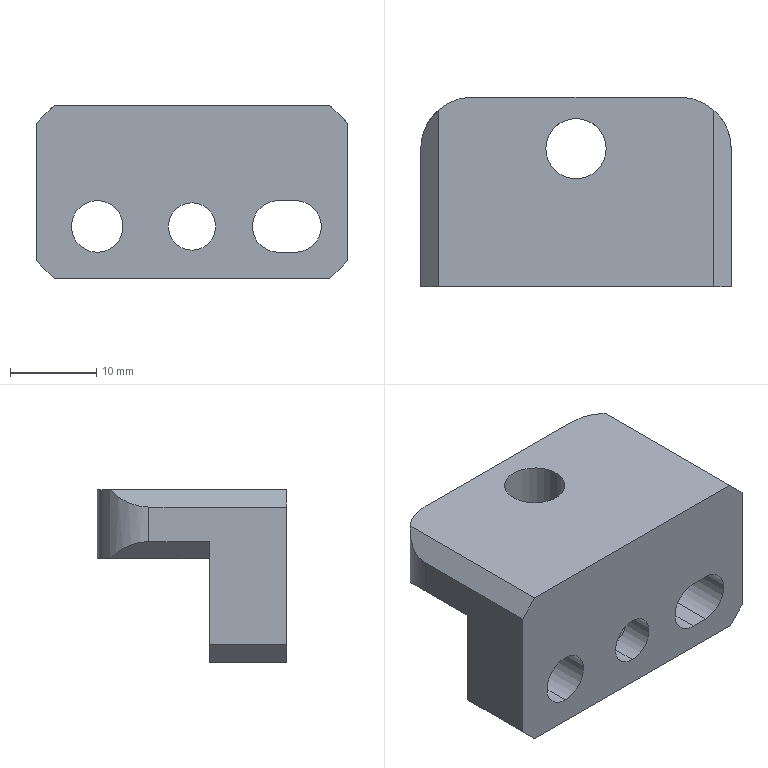Part | STEP file | QA-AD15 | 1 solid | 29 faces | box 36 x 22 x 20 mm | volume 8518 mm3 | plane 17 | cylinder 12 | commonest cylinder face diameters 6 x4 5.5 x2 7 x2 10 x2 12 x2